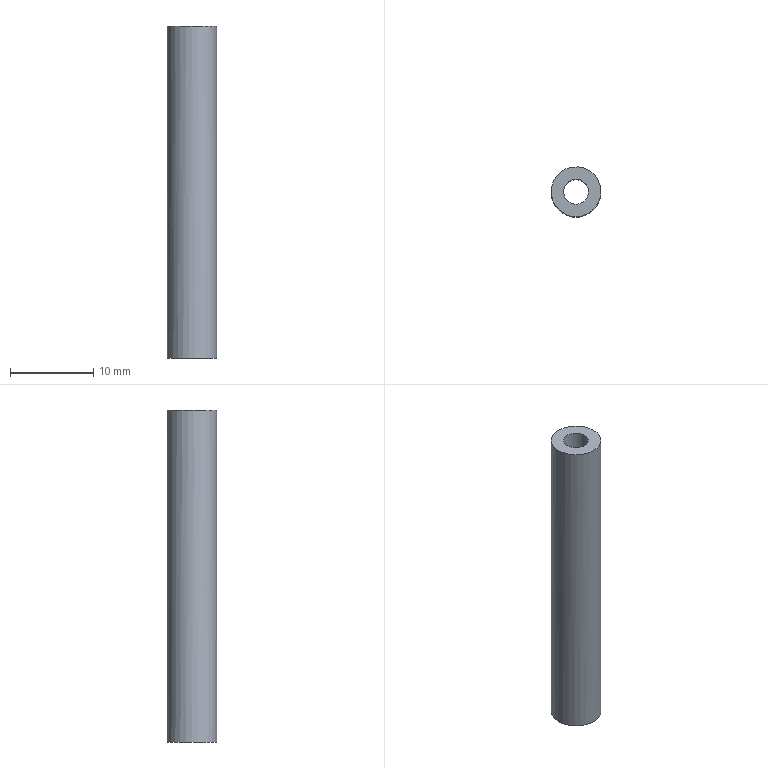Part | STEP file | gslz 2016.10.28-10_id3138_x_t | 1 solid | 4 faces | box 6 x 6 x 40 mm | volume 848.23 mm3 | cylinder 2 | plane 2 | commonest cylinder face diameters 3 x1 6 x1
STEP:
#1=CARTESIAN_POINT('',(0.,0.,0.));
#2=DIRECTION('',(0.,0.,1.));
#3=DIRECTION('',(1.,0.,0.));
#4=AXIS2_PLACEMENT_3D('',#1,#2,#3);
#5=CARTESIAN_POINT('',(-635.932,149.5,34.));
#6=VERTEX_POINT('',#5);
#7=CARTESIAN_POINT('',(-638.932,149.5,34.));
#8=DIRECTION('',(0.,0.,-1.));
#9=DIRECTION('',(1.,0.,0.));
#10=AXIS2_PLACEMENT_3D('',#7,#8,#9);
#11=CIRCLE('',#10,3.);
#12=CARTESIAN_POINT('',(-638.932,149.5,24.));
#13=DIRECTION('',(0.,0.,1.));
#14=DIRECTION('',(1.,0.,0.));
#15=AXIS2_PLACEMENT_3D('',#12,#13,#14);
#16=CYLINDRICAL_SURFACE('',#15,3.);
#17=CARTESIAN_POINT('',(6.283,10.));
#18=DIRECTION('',(-1.,0.));
#19=VECTOR('',#18,1.);
#20=LINE('',#17,#19);
#21=(GEOMETRIC_REPRESENTATION_CONTEXT(2)PARAMETRIC_REPRESENTATION_CONTEXT()REPRESENTATION_CONTEXT('',''));
#22=DEFINITIONAL_REPRESENTATION('',(#20),#21);
#23=PCURVE('',#16,#22);
#24=CARTESIAN_POINT('',(-638.932,149.5,34.));
#25=DIRECTION('',(0.,0.,1.));
#26=DIRECTION('',(1.,0.,0.));
#27=AXIS2_PLACEMENT_3D('',#24,#25,#26);
#28=PLANE('',#27);
#29=CARTESIAN_POINT('',(3.,0.));
#30=CARTESIAN_POINT('',(3.,-5.196));
#31=CARTESIAN_POINT('',(-1.5,-2.598));
#32=CARTESIAN_POINT('',(-6.,0.));
#33=CARTESIAN_POINT('',(-1.5,2.598));
#34=CARTESIAN_POINT('',(3.,5.196));
#35=CARTESIAN_POINT('',(3.,0.));
#36=(BOUNDED_CURVE()B_SPLINE_CURVE(2,(#29,#30,#31,#32,#33,#34,#35),.UNSPECIFIED.,.T.,.F.)B_SPLINE_CURVE_WITH_KNOTS((1,2,2,2,2,1),(-2.094,0.,2.094,4.189,6.283,8.378),.UNSPECIFIED.)CURVE()GEOMETRIC_REPRESENTATION_ITEM()RATIONAL_B_SPLINE_CURVE((1.,0.5,1.,0.5,1.,0.5,1.))REPRESENTATION_ITEM(''));
#37=(GEOMETRIC_REPRESENTATION_CONTEXT(2)PARAMETRIC_REPRESENTATION_CONTEXT()REPRESENTATION_CONTEXT('',''));
#38=DEFINITIONAL_REPRESENTATION('',(#36),#37);
#39=PCURVE('',#28,#38);
#40=SURFACE_CURVE('',#11,(#23,#39),.PCURVE_S1.);
#41=EDGE_CURVE('',#6,#6,#40,.T.);
#42=ORIENTED_EDGE('',*,*,#41,.F.);
#43=CARTESIAN_POINT('',(-635.932,149.5,74.));
#44=VERTEX_POINT('',#43);
#45=CARTESIAN_POINT('',(-635.932,149.5,34.));
#46=CARTESIAN_POINT('',(-635.932,149.5,74.));
#47=B_SPLINE_CURVE_WITH_KNOTS('',1,(#45,#46),.UNSPECIFIED.,.F.,.F.,(2,2),(10.,50.),.PIECEWISE_BEZIER_KNOTS.);
#48=CARTESIAN_POINT('',(6.283,0.));
#49=DIRECTION('',(0.,1.));
#50=VECTOR('',#49,1.);
#51=LINE('',#48,#50);
#52=(GEOMETRIC_REPRESENTATION_CONTEXT(2)PARAMETRIC_REPRESENTATION_CONTEXT()REPRESENTATION_CONTEXT('',''));
#53=DEFINITIONAL_REPRESENTATION('',(#51),#52);
#54=PCURVE('',#16,#53);
#55=CARTESIAN_POINT('',(0.,0.));
#56=DIRECTION('',(0.,1.));
#57=VECTOR('',#56,1.);
#58=LINE('',#55,#57);
#59=(GEOMETRIC_REPRESENTATION_CONTEXT(2)PARAMETRIC_REPRESENTATION_CONTEXT()REPRESENTATION_CONTEXT('',''));
#60=DEFINITIONAL_REPRESENTATION('',(#58),#59);
#61=PCURVE('',#16,#60);
#62=SEAM_CURVE('',#47,(#54,#61),.PCURVE_S1.);
#63=EDGE_CURVE('',#6,#44,#62,.T.);
#64=ORIENTED_EDGE('',*,*,#63,.T.);
#65=CARTESIAN_POINT('',(-638.932,146.5,74.));
#66=VERTEX_POINT('',#65);
#67=CARTESIAN_POINT('',(-638.932,149.5,74.));
#68=DIRECTION('',(0.,0.,-1.));
#69=DIRECTION('',(0.,-1.,0.));
#70=AXIS2_PLACEMENT_3D('',#67,#68,#69);
#71=CIRCLE('',#70,3.);
#72=CARTESIAN_POINT('',(10.996,50.));
#73=DIRECTION('',(-1.,0.));
#74=VECTOR('',#73,1.);
#75=LINE('',#72,#74);
#76=(GEOMETRIC_REPRESENTATION_CONTEXT(2)PARAMETRIC_REPRESENTATION_CONTEXT()REPRESENTATION_CONTEXT('',''));
#77=DEFINITIONAL_REPRESENTATION('',(#75),#76);
#78=PCURVE('',#16,#77);
#79=CARTESIAN_POINT('',(-576.515,124.515,74.));
#80=DIRECTION('',(0.,0.,1.));
#81=DIRECTION('',(0.,1.,0.));
#82=AXIS2_PLACEMENT_3D('',#79,#80,#81);
#83=PLANE('',#82);
#84=CARTESIAN_POINT('',(21.985,62.418));
#85=CARTESIAN_POINT('',(21.985,67.614));
#86=CARTESIAN_POINT('',(26.485,65.016));
#87=CARTESIAN_POINT('',(30.985,62.418));
#88=CARTESIAN_POINT('',(26.485,59.82));
#89=CARTESIAN_POINT('',(21.985,57.222));
#90=CARTESIAN_POINT('',(21.985,62.418));
#91=(BOUNDED_CURVE()B_SPLINE_CURVE(2,(#84,#85,#86,#87,#88,#89,#90),.UNSPECIFIED.,.T.,.F.)B_SPLINE_CURVE_WITH_KNOTS((1,2,2,2,2,1),(-2.094,0.,2.094,4.189,6.283,8.378),.UNSPECIFIED.)CURVE()GEOMETRIC_REPRESENTATION_ITEM()RATIONAL_B_SPLINE_CURVE((1.,0.5,1.,0.5,1.,0.5,1.))REPRESENTATION_ITEM(''));
#92=(GEOMETRIC_REPRESENTATION_CONTEXT(2)PARAMETRIC_REPRESENTATION_CONTEXT()REPRESENTATION_CONTEXT('',''));
#93=DEFINITIONAL_REPRESENTATION('',(#91),#92);
#94=PCURVE('',#83,#93);
#95=SURFACE_CURVE('',#71,(#78,#94),.PCURVE_S1.);
#96=EDGE_CURVE('',#44,#66,#95,.T.);
#97=ORIENTED_EDGE('',*,*,#96,.T.);
#98=CARTESIAN_POINT('',(-638.932,149.5,74.));
#99=DIRECTION('',(0.,0.,-1.));
#100=DIRECTION('',(0.,-1.,0.));
#101=AXIS2_PLACEMENT_3D('',#98,#99,#100);
#102=CIRCLE('',#101,3.);
#103=CARTESIAN_POINT('',(4.712,50.));
#104=DIRECTION('',(-1.,0.));
#105=VECTOR('',#104,1.);
#106=LINE('',#103,#105);
#107=(GEOMETRIC_REPRESENTATION_CONTEXT(2)PARAMETRIC_REPRESENTATION_CONTEXT()REPRESENTATION_CONTEXT('',''));
#108=DEFINITIONAL_REPRESENTATION('',(#106),#107);
#109=PCURVE('',#16,#108);
#110=CARTESIAN_POINT('',(21.985,62.418));
#111=CARTESIAN_POINT('',(21.985,67.614));
#112=CARTESIAN_POINT('',(26.485,65.016));
#113=CARTESIAN_POINT('',(30.985,62.418));
#114=CARTESIAN_POINT('',(26.485,59.82));
#115=CARTESIAN_POINT('',(21.985,57.222));
#116=CARTESIAN_POINT('',(21.985,62.418));
#117=(BOUNDED_CURVE()B_SPLINE_CURVE(2,(#110,#111,#112,#113,#114,#115,#116),.UNSPECIFIED.,.T.,.F.)B_SPLINE_CURVE_WITH_KNOTS((1,2,2,2,2,1),(-2.094,0.,2.094,4.189,6.283,8.378),.UNSPECIFIED.)CURVE()GEOMETRIC_REPRESENTATION_ITEM()RATIONAL_B_SPLINE_CURVE((1.,0.5,1.,0.5,1.,0.5,1.))REPRESENTATION_ITEM(''));
#118=(GEOMETRIC_REPRESENTATION_CONTEXT(2)PARAMETRIC_REPRESENTATION_CONTEXT()REPRESENTATION_CONTEXT('',''));
#119=DEFINITIONAL_REPRESENTATION('',(#117),#118);
#120=PCURVE('',#83,#119);
#121=SURFACE_CURVE('',#102,(#109,#120),.PCURVE_S1.);
#122=EDGE_CURVE('',#66,#44,#121,.T.);
#123=ORIENTED_EDGE('',*,*,#122,.T.);
#124=ORIENTED_EDGE('',*,*,#63,.F.);
#125=EDGE_LOOP('',(#42,#64,#97,#123,#124));
#126=FACE_BOUND('',#125,.T.);
#127=ADVANCED_FACE('',(#126),#16,.T.);
#128=CARTESIAN_POINT('',(-637.432,149.5,34.));
#129=VERTEX_POINT('',#128);
#130=CARTESIAN_POINT('',(-638.932,149.5,34.));
#131=DIRECTION('',(0.,0.,1.));
#132=DIRECTION('',(1.,0.,0.));
#133=AXIS2_PLACEMENT_3D('',#130,#131,#132);
#134=CIRCLE('',#133,1.5);
#135=CARTESIAN_POINT('',(0.,0.));
#136=DIRECTION('',(1.,0.));
#137=AXIS2_PLACEMENT_2D('',#135,#136);
#138=CIRCLE('',#137,1.5);
#139=(GEOMETRIC_REPRESENTATION_CONTEXT(2)PARAMETRIC_REPRESENTATION_CONTEXT()REPRESENTATION_CONTEXT('',''));
#140=DEFINITIONAL_REPRESENTATION('',(#138),#139);
#141=PCURVE('',#28,#140);
#142=CARTESIAN_POINT('',(-638.932,149.5,114.));
#143=DIRECTION('',(0.,0.,-1.));
#144=DIRECTION('',(1.,0.,0.));
#145=AXIS2_PLACEMENT_3D('',#142,#143,#144);
#146=CYLINDRICAL_SURFACE('',#145,1.5);
#147=CARTESIAN_POINT('',(6.283,80.));
#148=DIRECTION('',(-1.,0.));
#149=VECTOR('',#148,1.);
#150=LINE('',#147,#149);
#151=(GEOMETRIC_REPRESENTATION_CONTEXT(2)PARAMETRIC_REPRESENTATION_CONTEXT()REPRESENTATION_CONTEXT('',''));
#152=DEFINITIONAL_REPRESENTATION('',(#150),#151);
#153=PCURVE('',#146,#152);
#154=SURFACE_CURVE('',#134,(#141,#153),.PCURVE_S1.);
#155=EDGE_CURVE('',#129,#129,#154,.T.);
#156=ORIENTED_EDGE('',*,*,#155,.T.);
#157=EDGE_LOOP('',(#156));
#158=FACE_BOUND('',#157,.T.);
#159=ORIENTED_EDGE('',*,*,#41,.T.);
#160=EDGE_LOOP('',(#159));
#161=FACE_BOUND('',#160,.T.);
#162=ADVANCED_FACE('',(#158,#161),#28,.F.);
#163=CARTESIAN_POINT('',(-638.932,148.,74.));
#164=VERTEX_POINT('',#163);
#165=CARTESIAN_POINT('',(-637.432,149.5,74.));
#166=VERTEX_POINT('',#165);
#167=CARTESIAN_POINT('',(-638.932,149.5,74.));
#168=DIRECTION('',(0.,0.,1.));
#169=DIRECTION('',(0.,-1.,0.));
#170=AXIS2_PLACEMENT_3D('',#167,#168,#169);
#171=CIRCLE('',#170,1.5);
#172=CARTESIAN_POINT('',(24.985,62.418));
#173=DIRECTION('',(-1.,0.));
#174=AXIS2_PLACEMENT_2D('',#172,#173);
#175=CIRCLE('',#174,1.5);
#176=(GEOMETRIC_REPRESENTATION_CONTEXT(2)PARAMETRIC_REPRESENTATION_CONTEXT()REPRESENTATION_CONTEXT('',''));
#177=DEFINITIONAL_REPRESENTATION('',(#175),#176);
#178=PCURVE('',#83,#177);
#179=CARTESIAN_POINT('',(1.571,40.));
#180=DIRECTION('',(-1.,0.));
#181=VECTOR('',#180,1.);
#182=LINE('',#179,#181);
#183=(GEOMETRIC_REPRESENTATION_CONTEXT(2)PARAMETRIC_REPRESENTATION_CONTEXT()REPRESENTATION_CONTEXT('',''));
#184=DEFINITIONAL_REPRESENTATION('',(#182),#183);
#185=PCURVE('',#146,#184);
#186=SURFACE_CURVE('',#171,(#178,#185),.PCURVE_S1.);
#187=EDGE_CURVE('',#164,#166,#186,.T.);
#188=ORIENTED_EDGE('',*,*,#187,.F.);
#189=CARTESIAN_POINT('',(-638.932,149.5,74.));
#190=DIRECTION('',(0.,0.,1.));
#191=DIRECTION('',(0.,-1.,0.));
#192=AXIS2_PLACEMENT_3D('',#189,#190,#191);
#193=CIRCLE('',#192,1.5);
#194=CARTESIAN_POINT('',(24.985,62.418));
#195=DIRECTION('',(-1.,0.));
#196=AXIS2_PLACEMENT_2D('',#194,#195);
#197=CIRCLE('',#196,1.5);
#198=(GEOMETRIC_REPRESENTATION_CONTEXT(2)PARAMETRIC_REPRESENTATION_CONTEXT()REPRESENTATION_CONTEXT('',''));
#199=DEFINITIONAL_REPRESENTATION('',(#197),#198);
#200=PCURVE('',#83,#199);
#201=CARTESIAN_POINT('',(7.854,40.));
#202=DIRECTION('',(-1.,0.));
#203=VECTOR('',#202,1.);
#204=LINE('',#201,#203);
#205=(GEOMETRIC_REPRESENTATION_CONTEXT(2)PARAMETRIC_REPRESENTATION_CONTEXT()REPRESENTATION_CONTEXT('',''));
#206=DEFINITIONAL_REPRESENTATION('',(#204),#205);
#207=PCURVE('',#146,#206);
#208=SURFACE_CURVE('',#193,(#200,#207),.PCURVE_S1.);
#209=EDGE_CURVE('',#166,#164,#208,.T.);
#210=ORIENTED_EDGE('',*,*,#209,.F.);
#211=EDGE_LOOP('',(#188,#210));
#212=FACE_BOUND('',#211,.T.);
#213=ORIENTED_EDGE('',*,*,#122,.F.);
#214=ORIENTED_EDGE('',*,*,#96,.F.);
#215=EDGE_LOOP('',(#213,#214));
#216=FACE_BOUND('',#215,.T.);
#217=ADVANCED_FACE('',(#212,#216),#83,.T.);
#218=ORIENTED_EDGE('',*,*,#209,.F.);
#219=CARTESIAN_POINT('',(-637.432,149.5,74.));
#220=CARTESIAN_POINT('',(-637.432,149.5,34.));
#221=B_SPLINE_CURVE_WITH_KNOTS('',1,(#219,#220),.UNSPECIFIED.,.F.,.F.,(2,2),(40.,80.),.PIECEWISE_BEZIER_KNOTS.);
#222=CARTESIAN_POINT('',(6.283,0.));
#223=DIRECTION('',(0.,1.));
#224=VECTOR('',#223,1.);
#225=LINE('',#222,#224);
#226=(GEOMETRIC_REPRESENTATION_CONTEXT(2)PARAMETRIC_REPRESENTATION_CONTEXT()REPRESENTATION_CONTEXT('',''));
#227=DEFINITIONAL_REPRESENTATION('',(#225),#226);
#228=PCURVE('',#146,#227);
#229=CARTESIAN_POINT('',(0.,0.));
#230=DIRECTION('',(0.,1.));
#231=VECTOR('',#230,1.);
#232=LINE('',#229,#231);
#233=(GEOMETRIC_REPRESENTATION_CONTEXT(2)PARAMETRIC_REPRESENTATION_CONTEXT()REPRESENTATION_CONTEXT('',''));
#234=DEFINITIONAL_REPRESENTATION('',(#232),#233);
#235=PCURVE('',#146,#234);
#236=SEAM_CURVE('',#221,(#228,#235),.PCURVE_S1.);
#237=EDGE_CURVE('',#166,#129,#236,.T.);
#238=ORIENTED_EDGE('',*,*,#237,.T.);
#239=ORIENTED_EDGE('',*,*,#155,.T.);
#240=ORIENTED_EDGE('',*,*,#237,.F.);
#241=ORIENTED_EDGE('',*,*,#187,.F.);
#242=EDGE_LOOP('',(#218,#238,#239,#240,#241));
#243=FACE_BOUND('',#242,.F.);
#244=ADVANCED_FACE('',(#243),#146,.F.);
#245=CLOSED_SHELL('',(#127,#162,#217,#244));
#246=MANIFOLD_SOLID_BREP('',#245);
#247=(LENGTH_UNIT()NAMED_UNIT(*)SI_UNIT(.MILLI.,.METRE.));
#248=UNCERTAINTY_MEASURE_WITH_UNIT(LENGTH_MEASURE(0.000005),#247,'','');
#249=(NAMED_UNIT(*)PLANE_ANGLE_UNIT()SI_UNIT($,.RADIAN.));
#250=(NAMED_UNIT(*)SI_UNIT($,.STERADIAN.)SOLID_ANGLE_UNIT());
#251=(GEOMETRIC_REPRESENTATION_CONTEXT(3)GLOBAL_UNCERTAINTY_ASSIGNED_CONTEXT((#248))GLOBAL_UNIT_ASSIGNED_CONTEXT((#247,#249,#250))REPRESENTATION_CONTEXT('',''));
#252=ADVANCED_BREP_SHAPE_REPRESENTATION('',(#4,#246),#251);